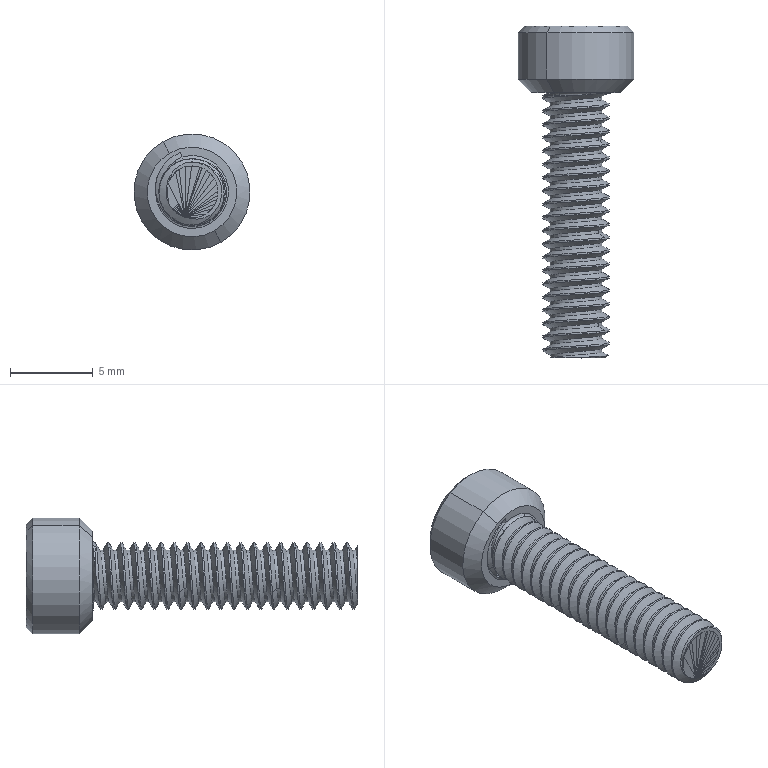Part | NX | features BREP 1 | 1 solid | 93 faces | box 7 x 20 x 7 mm | volume 280.839 mm3 | cylinder 45 | spline 21 | plane 16 | cone 8 | torus 3 | commonest cylinder face diameters 4 x41 4.173 x2 7 x2